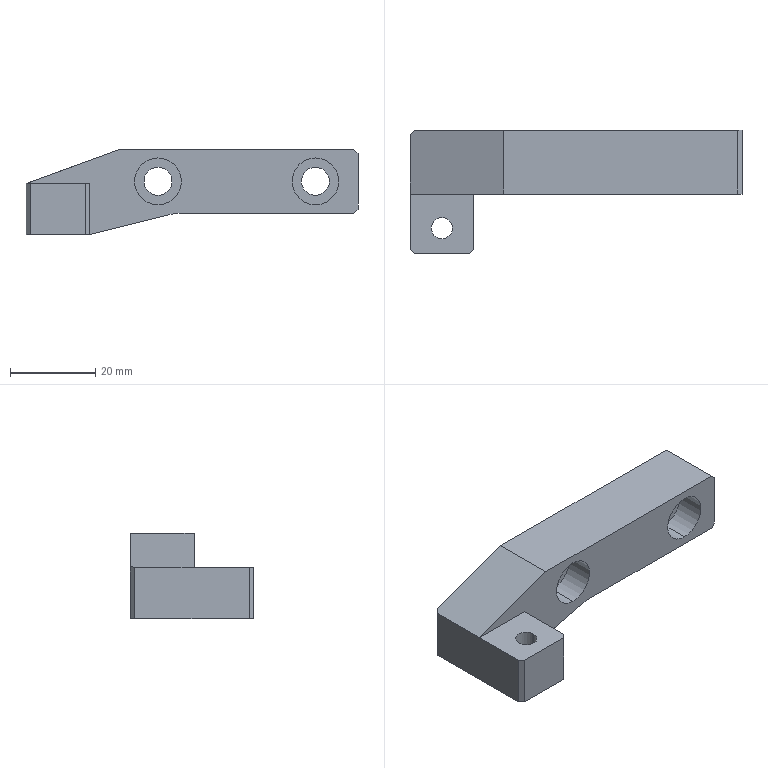Part | SolidWorks | features ICE 3, HoleWzd 2, Chamfer 1, Extrusion 1, Fillet 1 | 1 solid | 30 faces | box 78 x 29 x 20 mm | volume 18504 mm3 | plane 19 | cylinder 11 | commonest cylinder face diameters 6.6 x4 11 x4 5 x2 20 x1
STEP:
#1=CARTESIAN_POINT('',(-34.,-15.5,-12.5));
#2=VERTEX_POINT('',#1);
#3=CARTESIAN_POINT('',(-29.,-15.5,-12.5));
#4=VERTEX_POINT('',#3);
#5=CARTESIAN_POINT('',(-31.5,-15.5,-12.5));
#6=DIRECTION('',(0.,0.,1.));
#7=DIRECTION('',(1.,0.,0.));
#8=AXIS2_PLACEMENT_3D('',#5,#6,#7);
#9=CIRCLE('',#8,2.5);
#10=EDGE_CURVE('',#2,#4,#9,.T.);
#11=ORIENTED_EDGE('',*,*,#10,.F.);
#12=CARTESIAN_POINT('',(-34.,-15.5,-0.5));
#13=VERTEX_POINT('',#12);
#14=CARTESIAN_POINT('',(-34.,-15.5,-0.5));
#15=DIRECTION('',(0.,0.,1.));
#16=VECTOR('',#15,1000.);
#17=LINE('',#14,#16);
#18=EDGE_CURVE('',#2,#13,#17,.T.);
#19=ORIENTED_EDGE('',*,*,#18,.T.);
#20=CARTESIAN_POINT('',(-29.,-15.5,-0.5));
#21=VERTEX_POINT('',#20);
#22=CARTESIAN_POINT('',(-31.5,-15.5,-0.5));
#23=DIRECTION('',(0.,0.,1.));
#24=DIRECTION('',(1.,0.,0.));
#25=AXIS2_PLACEMENT_3D('',#22,#23,#24);
#26=CIRCLE('',#25,2.5);
#27=EDGE_CURVE('',#13,#21,#26,.T.);
#28=ORIENTED_EDGE('',*,*,#27,.T.);
#29=CARTESIAN_POINT('',(-29.,-15.5,-0.5));
#30=DIRECTION('',(0.,0.,1.));
#31=VECTOR('',#30,1000.);
#32=LINE('',#29,#31);
#33=EDGE_CURVE('',#4,#21,#32,.T.);
#34=ORIENTED_EDGE('',*,*,#33,.F.);
#35=EDGE_LOOP('',(#11,#19,#28,#34));
#36=FACE_OUTER_BOUND('',#35,.T.);
#37=CARTESIAN_POINT('',(-31.5,-15.5,-0.5));
#38=DIRECTION('',(0.,0.,1.));
#39=DIRECTION('',(1.,0.,0.));
#40=AXIS2_PLACEMENT_3D('',#37,#38,#39);
#41=CYLINDRICAL_SURFACE('',#40,2.5);
#42=ADVANCED_FACE('',(#36),#41,.F.);
#43=CARTESIAN_POINT('',(29.,-0.7,5.5));
#44=VERTEX_POINT('',#43);
#45=CARTESIAN_POINT('',(29.,-0.7,-5.5));
#46=VERTEX_POINT('',#45);
#47=CARTESIAN_POINT('',(29.,-0.7,0.));
#48=DIRECTION('',(0.,-1.,0.));
#49=DIRECTION('',(0.,0.,-1.));
#50=AXIS2_PLACEMENT_3D('',#47,#48,#49);
#51=CIRCLE('',#50,5.5);
#52=EDGE_CURVE('',#44,#46,#51,.T.);
#53=ORIENTED_EDGE('',*,*,#52,.F.);
#54=CARTESIAN_POINT('',(29.,-7.5,5.5));
#55=VERTEX_POINT('',#54);
#56=CARTESIAN_POINT('',(29.,-7.5,5.5));
#57=DIRECTION('',(0.,-1.,0.));
#58=VECTOR('',#57,1000.);
#59=LINE('',#56,#58);
#60=EDGE_CURVE('',#44,#55,#59,.T.);
#61=ORIENTED_EDGE('',*,*,#60,.T.);
#62=CARTESIAN_POINT('',(29.,-7.5,-5.5));
#63=VERTEX_POINT('',#62);
#64=CARTESIAN_POINT('',(29.,-7.5,0.));
#65=DIRECTION('',(0.,-1.,0.));
#66=DIRECTION('',(0.,0.,-1.));
#67=AXIS2_PLACEMENT_3D('',#64,#65,#66);
#68=CIRCLE('',#67,5.5);
#69=EDGE_CURVE('',#55,#63,#68,.T.);
#70=ORIENTED_EDGE('',*,*,#69,.T.);
#71=CARTESIAN_POINT('',(29.,-7.5,-5.5));
#72=DIRECTION('',(0.,-1.,0.));
#73=VECTOR('',#72,1000.);
#74=LINE('',#71,#73);
#75=EDGE_CURVE('',#46,#63,#74,.T.);
#76=ORIENTED_EDGE('',*,*,#75,.F.);
#77=EDGE_LOOP('',(#53,#61,#70,#76));
#78=FACE_OUTER_BOUND('',#77,.T.);
#79=CARTESIAN_POINT('',(29.,-7.5,0.));
#80=DIRECTION('',(0.,-1.,0.));
#81=DIRECTION('',(0.,0.,-1.));
#82=AXIS2_PLACEMENT_3D('',#79,#80,#81);
#83=CYLINDRICAL_SURFACE('',#82,5.5);
#84=ADVANCED_FACE('',(#78),#83,.F.);
#85=CARTESIAN_POINT('',(29.,7.5,3.3));
#86=VERTEX_POINT('',#85);
#87=CARTESIAN_POINT('',(29.,7.5,-3.3));
#88=VERTEX_POINT('',#87);
#89=CARTESIAN_POINT('',(29.,7.5,0.));
#90=DIRECTION('',(0.,-1.,0.));
#91=DIRECTION('',(0.,0.,-1.));
#92=AXIS2_PLACEMENT_3D('',#89,#90,#91);
#93=CIRCLE('',#92,3.3);
#94=EDGE_CURVE('',#86,#88,#93,.T.);
#95=ORIENTED_EDGE('',*,*,#94,.F.);
#96=CARTESIAN_POINT('',(29.,-0.7,3.3));
#97=VERTEX_POINT('',#96);
#98=CARTESIAN_POINT('',(29.,-7.5,3.3));
#99=DIRECTION('',(0.,-1.,0.));
#100=VECTOR('',#99,1000.);
#101=LINE('',#98,#100);
#102=EDGE_CURVE('',#86,#97,#101,.T.);
#103=ORIENTED_EDGE('',*,*,#102,.T.);
#104=CARTESIAN_POINT('',(29.,-0.7,-3.3));
#105=VERTEX_POINT('',#104);
#106=CARTESIAN_POINT('',(29.,-0.7,0.));
#107=DIRECTION('',(0.,-1.,0.));
#108=DIRECTION('',(0.,0.,-1.));
#109=AXIS2_PLACEMENT_3D('',#106,#107,#108);
#110=CIRCLE('',#109,3.3);
#111=EDGE_CURVE('',#97,#105,#110,.T.);
#112=ORIENTED_EDGE('',*,*,#111,.T.);
#113=CARTESIAN_POINT('',(29.,-7.5,-3.3));
#114=DIRECTION('',(0.,-1.,0.));
#115=VECTOR('',#114,1000.);
#116=LINE('',#113,#115);
#117=EDGE_CURVE('',#88,#105,#116,.T.);
#118=ORIENTED_EDGE('',*,*,#117,.F.);
#119=EDGE_LOOP('',(#95,#103,#112,#118));
#120=FACE_OUTER_BOUND('',#119,.T.);
#121=CARTESIAN_POINT('',(29.,-7.5,0.));
#122=DIRECTION('',(0.,-1.,0.));
#123=DIRECTION('',(0.,0.,-1.));
#124=AXIS2_PLACEMENT_3D('',#121,#122,#123);
#125=CYLINDRICAL_SURFACE('',#124,3.3);
#126=ADVANCED_FACE('',(#120),#125,.F.);
#127=CARTESIAN_POINT('',(-8.,-0.7,5.5));
#128=VERTEX_POINT('',#127);
#129=CARTESIAN_POINT('',(-8.,-0.7,-5.5));
#130=VERTEX_POINT('',#129);
#131=CARTESIAN_POINT('',(-8.,-0.7,0.));
#132=DIRECTION('',(0.,-1.,0.));
#133=DIRECTION('',(0.,0.,-1.));
#134=AXIS2_PLACEMENT_3D('',#131,#132,#133);
#135=CIRCLE('',#134,5.5);
#136=EDGE_CURVE('',#128,#130,#135,.T.);
#137=ORIENTED_EDGE('',*,*,#136,.F.);
#138=CARTESIAN_POINT('',(-8.,-7.5,5.5));
#139=VERTEX_POINT('',#138);
#140=CARTESIAN_POINT('',(-8.,-7.5,5.5));
#141=DIRECTION('',(0.,-1.,0.));
#142=VECTOR('',#141,1000.);
#143=LINE('',#140,#142);
#144=EDGE_CURVE('',#128,#139,#143,.T.);
#145=ORIENTED_EDGE('',*,*,#144,.T.);
#146=CARTESIAN_POINT('',(-8.,-7.5,-5.5));
#147=VERTEX_POINT('',#146);
#148=CARTESIAN_POINT('',(-8.,-7.5,0.));
#149=DIRECTION('',(0.,-1.,0.));
#150=DIRECTION('',(0.,0.,-1.));
#151=AXIS2_PLACEMENT_3D('',#148,#149,#150);
#152=CIRCLE('',#151,5.5);
#153=EDGE_CURVE('',#139,#147,#152,.T.);
#154=ORIENTED_EDGE('',*,*,#153,.T.);
#155=CARTESIAN_POINT('',(-8.,-7.5,-5.5));
#156=DIRECTION('',(0.,-1.,0.));
#157=VECTOR('',#156,1000.);
#158=LINE('',#155,#157);
#159=EDGE_CURVE('',#130,#147,#158,.T.);
#160=ORIENTED_EDGE('',*,*,#159,.F.);
#161=EDGE_LOOP('',(#137,#145,#154,#160));
#162=FACE_OUTER_BOUND('',#161,.T.);
#163=CARTESIAN_POINT('',(-8.,-7.5,0.));
#164=DIRECTION('',(0.,-1.,0.));
#165=DIRECTION('',(0.,0.,-1.));
#166=AXIS2_PLACEMENT_3D('',#163,#164,#165);
#167=CYLINDRICAL_SURFACE('',#166,5.5);
#168=ADVANCED_FACE('',(#162),#167,.F.);
#169=CARTESIAN_POINT('',(-8.,7.5,3.3));
#170=VERTEX_POINT('',#169);
#171=CARTESIAN_POINT('',(-8.,7.5,-3.3));
#172=VERTEX_POINT('',#171);
#173=CARTESIAN_POINT('',(-8.,7.5,0.));
#174=DIRECTION('',(0.,-1.,0.));
#175=DIRECTION('',(0.,0.,-1.));
#176=AXIS2_PLACEMENT_3D('',#173,#174,#175);
#177=CIRCLE('',#176,3.3);
#178=EDGE_CURVE('',#170,#172,#177,.T.);
#179=ORIENTED_EDGE('',*,*,#178,.F.);
#180=CARTESIAN_POINT('',(-8.,-0.7,3.3));
#181=VERTEX_POINT('',#180);
#182=CARTESIAN_POINT('',(-8.,-7.5,3.3));
#183=DIRECTION('',(0.,-1.,0.));
#184=VECTOR('',#183,1000.);
#185=LINE('',#182,#184);
#186=EDGE_CURVE('',#170,#181,#185,.T.);
#187=ORIENTED_EDGE('',*,*,#186,.T.);
#188=CARTESIAN_POINT('',(-8.,-0.7,-3.3));
#189=VERTEX_POINT('',#188);
#190=CARTESIAN_POINT('',(-8.,-0.7,0.));
#191=DIRECTION('',(0.,-1.,0.));
#192=DIRECTION('',(0.,0.,-1.));
#193=AXIS2_PLACEMENT_3D('',#190,#191,#192);
#194=CIRCLE('',#193,3.3);
#195=EDGE_CURVE('',#181,#189,#194,.T.);
#196=ORIENTED_EDGE('',*,*,#195,.T.);
#197=CARTESIAN_POINT('',(-8.,-7.5,-3.3));
#198=DIRECTION('',(0.,-1.,0.));
#199=VECTOR('',#198,1000.);
#200=LINE('',#197,#199);
#201=EDGE_CURVE('',#172,#189,#200,.T.);
#202=ORIENTED_EDGE('',*,*,#201,.F.);
#203=EDGE_LOOP('',(#179,#187,#196,#202));
#204=FACE_OUTER_BOUND('',#203,.T.);
#205=CARTESIAN_POINT('',(-8.,-7.5,0.));
#206=DIRECTION('',(0.,-1.,0.));
#207=DIRECTION('',(0.,0.,-1.));
#208=AXIS2_PLACEMENT_3D('',#205,#206,#207);
#209=CYLINDRICAL_SURFACE('',#208,3.3);
#210=ADVANCED_FACE('',(#204),#209,.F.);
#211=CARTESIAN_POINT('',(38.,-7.5,-7.5));
#212=VERTEX_POINT('',#211);
#213=CARTESIAN_POINT('',(-2.769,-7.5,-7.5));
#214=VERTEX_POINT('',#213);
#215=CARTESIAN_POINT('',(-39.,-7.5,-7.5));
#216=DIRECTION('',(-1.,0.,0.));
#217=VECTOR('',#216,1000.);
#218=LINE('',#215,#217);
#219=EDGE_CURVE('',#212,#214,#218,.T.);
#220=ORIENTED_EDGE('',*,*,#219,.F.);
#221=CARTESIAN_POINT('',(39.,-7.5,-6.5));
#222=VERTEX_POINT('',#221);
#223=CARTESIAN_POINT('',(22.75,-7.5,-22.75));
#224=DIRECTION('',(0.7071,0.,0.7071));
#225=VECTOR('',#224,1000.);
#226=LINE('',#223,#225);
#227=EDGE_CURVE('',#212,#222,#226,.T.);
#228=ORIENTED_EDGE('',*,*,#227,.T.);
#229=CARTESIAN_POINT('',(39.,-7.5,6.5));
#230=VERTEX_POINT('',#229);
#231=CARTESIAN_POINT('',(39.,-7.5,7.5));
#232=DIRECTION('',(0.,0.,-1.));
#233=VECTOR('',#232,1000.);
#234=LINE('',#231,#233);
#235=EDGE_CURVE('',#230,#222,#234,.T.);
#236=ORIENTED_EDGE('',*,*,#235,.F.);
#237=CARTESIAN_POINT('',(38.,-7.5,7.5));
#238=VERTEX_POINT('',#237);
#239=CARTESIAN_POINT('',(22.75,-7.5,22.75));
#240=DIRECTION('',(-0.7071,0.,0.7071));
#241=VECTOR('',#240,1000.);
#242=LINE('',#239,#241);
#243=EDGE_CURVE('',#230,#238,#242,.T.);
#244=ORIENTED_EDGE('',*,*,#243,.T.);
#245=CARTESIAN_POINT('',(-17.,-7.5,7.5));
#246=VERTEX_POINT('',#245);
#247=CARTESIAN_POINT('',(-39.,-7.5,7.5));
#248=DIRECTION('',(1.,0.,0.));
#249=VECTOR('',#248,1000.);
#250=LINE('',#247,#249);
#251=EDGE_CURVE('',#246,#238,#250,.T.);
#252=ORIENTED_EDGE('',*,*,#251,.F.);
#253=CARTESIAN_POINT('',(-39.,-7.5,-0.5));
#254=VERTEX_POINT('',#253);
#255=CARTESIAN_POINT('',(-4.394,-7.5,12.084));
#256=DIRECTION('',(0.9398,0.,0.3417));
#257=VECTOR('',#256,1000.);
#258=LINE('',#255,#257);
#259=EDGE_CURVE('',#254,#246,#258,.T.);
#260=ORIENTED_EDGE('',*,*,#259,.F.);
#261=CARTESIAN_POINT('',(-24.,-7.5,-0.5));
#262=VERTEX_POINT('',#261);
#263=CARTESIAN_POINT('',(-39.,-7.5,-0.5));
#264=DIRECTION('',(1.,0.,0.));
#265=VECTOR('',#264,1000.);
#266=LINE('',#263,#265);
#267=EDGE_CURVE('',#254,#262,#266,.T.);
#268=ORIENTED_EDGE('',*,*,#267,.T.);
#269=CARTESIAN_POINT('',(-24.,-7.5,-12.5));
#270=VERTEX_POINT('',#269);
#271=CARTESIAN_POINT('',(-24.,-7.5,-12.5));
#272=DIRECTION('',(0.,0.,-1.));
#273=VECTOR('',#272,1000.);
#274=LINE('',#271,#273);
#275=EDGE_CURVE('',#262,#270,#274,.T.);
#276=ORIENTED_EDGE('',*,*,#275,.T.);
#277=CARTESIAN_POINT('',(-5.194,-7.5,-7.799));
#278=VERTEX_POINT('',#277);
#279=CARTESIAN_POINT('',(-4.,-7.5,-7.5));
#280=DIRECTION('',(-0.9701,0.,-0.2425));
#281=VECTOR('',#280,1000.);
#282=LINE('',#279,#281);
#283=EDGE_CURVE('',#278,#270,#282,.T.);
#284=ORIENTED_EDGE('',*,*,#283,.F.);
#285=CARTESIAN_POINT('',(-2.769,-7.5,-17.5));
#286=DIRECTION('',(0.,1.,0.));
#287=DIRECTION('',(0.,0.,-1.));
#288=AXIS2_PLACEMENT_3D('',#285,#286,#287);
#289=CIRCLE('',#288,10.);
#290=EDGE_CURVE('',#278,#214,#289,.T.);
#291=ORIENTED_EDGE('',*,*,#290,.T.);
#292=EDGE_LOOP('',(#220,#228,#236,#244,#252,#260,#268,#276,#284,#291));
#293=FACE_OUTER_BOUND('',#292,.T.);
#294=CARTESIAN_POINT('',(29.,-7.5,0.));
#295=DIRECTION('',(0.,-1.,0.));
#296=DIRECTION('',(0.,0.,-1.));
#297=AXIS2_PLACEMENT_3D('',#294,#295,#296);
#298=CIRCLE('',#297,5.5);
#299=EDGE_CURVE('',#63,#55,#298,.T.);
#300=ORIENTED_EDGE('',*,*,#299,.F.);
#301=ORIENTED_EDGE('',*,*,#69,.F.);
#302=EDGE_LOOP('',(#300,#301));
#303=FACE_BOUND('',#302,.T.);
#304=CARTESIAN_POINT('',(-8.,-7.5,0.));
#305=DIRECTION('',(0.,-1.,0.));
#306=DIRECTION('',(0.,0.,-1.));
#307=AXIS2_PLACEMENT_3D('',#304,#305,#306);
#308=CIRCLE('',#307,5.5);
#309=EDGE_CURVE('',#147,#139,#308,.T.);
#310=ORIENTED_EDGE('',*,*,#309,.F.);
#311=ORIENTED_EDGE('',*,*,#153,.F.);
#312=EDGE_LOOP('',(#310,#311));
#313=FACE_BOUND('',#312,.T.);
#314=CARTESIAN_POINT('',(0.,-7.5,0.));
#315=DIRECTION('',(0.,-1.,0.));
#316=DIRECTION('',(0.,0.,-1.));
#317=AXIS2_PLACEMENT_3D('',#314,#315,#316);
#318=PLANE('',#317);
#319=ADVANCED_FACE('',(#293,#303,#313),#318,.T.);
#320=ORIENTED_EDGE('',*,*,#235,.T.);
#321=CARTESIAN_POINT('',(39.,7.5,-6.5));
#322=VERTEX_POINT('',#321);
#323=CARTESIAN_POINT('',(39.,7.5,-6.5));
#324=DIRECTION('',(0.,1.,0.));
#325=VECTOR('',#324,1000.);
#326=LINE('',#323,#325);
#327=EDGE_CURVE('',#222,#322,#326,.T.);
#328=ORIENTED_EDGE('',*,*,#327,.T.);
#329=CARTESIAN_POINT('',(39.,7.5,6.5));
#330=VERTEX_POINT('',#329);
#331=CARTESIAN_POINT('',(39.,7.5,7.5));
#332=DIRECTION('',(0.,0.,-1.));
#333=VECTOR('',#332,1000.);
#334=LINE('',#331,#333);
#335=EDGE_CURVE('',#330,#322,#334,.T.);
#336=ORIENTED_EDGE('',*,*,#335,.F.);
#337=CARTESIAN_POINT('',(39.,7.5,6.5));
#338=DIRECTION('',(0.,-1.,0.));
#339=VECTOR('',#338,1000.);
#340=LINE('',#337,#339);
#341=EDGE_CURVE('',#330,#230,#340,.T.);
#342=ORIENTED_EDGE('',*,*,#341,.T.);
#343=EDGE_LOOP('',(#320,#328,#336,#342));
#344=FACE_OUTER_BOUND('',#343,.T.);
#345=CARTESIAN_POINT('',(39.,7.5,7.5));
#346=DIRECTION('',(-1.,0.,0.));
#347=DIRECTION('',(0.,0.,1.));
#348=AXIS2_PLACEMENT_3D('',#345,#346,#347);
#349=PLANE('',#348);
#350=ADVANCED_FACE('',(#344),#349,.F.);
#351=ORIENTED_EDGE('',*,*,#219,.T.);
#352=CARTESIAN_POINT('',(-2.769,7.5,-7.5));
#353=VERTEX_POINT('',#352);
#354=CARTESIAN_POINT('',(-2.769,7.5,-7.5));
#355=DIRECTION('',(0.,1.,0.));
#356=VECTOR('',#355,1000.);
#357=LINE('',#354,#356);
#358=EDGE_CURVE('',#214,#353,#357,.T.);
#359=ORIENTED_EDGE('',*,*,#358,.T.);
#360=CARTESIAN_POINT('',(38.,7.5,-7.5));
#361=VERTEX_POINT('',#360);
#362=CARTESIAN_POINT('',(-39.,7.5,-7.5));
#363=DIRECTION('',(-1.,0.,0.));
#364=VECTOR('',#363,1000.);
#365=LINE('',#362,#364);
#366=EDGE_CURVE('',#361,#353,#365,.T.);
#367=ORIENTED_EDGE('',*,*,#366,.F.);
#368=CARTESIAN_POINT('',(38.,7.5,-7.5));
#369=DIRECTION('',(0.,-1.,0.));
#370=VECTOR('',#369,1000.);
#371=LINE('',#368,#370);
#372=EDGE_CURVE('',#361,#212,#371,.T.);
#373=ORIENTED_EDGE('',*,*,#372,.T.);
#374=EDGE_LOOP('',(#351,#359,#367,#373));
#375=FACE_OUTER_BOUND('',#374,.T.);
#376=CARTESIAN_POINT('',(-39.,7.5,-7.5));
#377=DIRECTION('',(0.,0.,1.));
#378=DIRECTION('',(1.,0.,0.));
#379=AXIS2_PLACEMENT_3D('',#376,#377,#378);
#380=PLANE('',#379);
#381=ADVANCED_FACE('',(#375),#380,.F.);
#382=CARTESIAN_POINT('',(-39.,6.5,-0.5));
#383=VERTEX_POINT('',#382);
#384=CARTESIAN_POINT('',(-39.,7.5,-0.5));
#385=DIRECTION('',(0.,-1.,0.));
#386=VECTOR('',#385,1000.);
#387=LINE('',#384,#386);
#388=EDGE_CURVE('',#383,#254,#387,.T.);
#389=ORIENTED_EDGE('',*,*,#388,.F.);
#390=CARTESIAN_POINT('',(-39.,6.5,-12.5));
#391=VERTEX_POINT('',#390);
#392=CARTESIAN_POINT('',(-39.,6.5,7.5));
#393=DIRECTION('',(0.,0.,-1.));
#394=VECTOR('',#393,1000.);
#395=LINE('',#392,#394);
#396=EDGE_CURVE('',#383,#391,#395,.T.);
#397=ORIENTED_EDGE('',*,*,#396,.T.);
#398=CARTESIAN_POINT('',(-39.,-20.5,-12.5));
#399=VERTEX_POINT('',#398);
#400=CARTESIAN_POINT('',(-39.,-42.855,-12.5));
#401=DIRECTION('',(0.,1.,0.));
#402=VECTOR('',#401,1000.);
#403=LINE('',#400,#402);
#404=EDGE_CURVE('',#399,#391,#403,.T.);
#405=ORIENTED_EDGE('',*,*,#404,.F.);
#406=CARTESIAN_POINT('',(-39.,-20.5,-0.5));
#407=VERTEX_POINT('',#406);
#408=CARTESIAN_POINT('',(-39.,-20.5,7.5));
#409=DIRECTION('',(0.,0.,1.));
#410=VECTOR('',#409,1000.);
#411=LINE('',#408,#410);
#412=EDGE_CURVE('',#399,#407,#411,.T.);
#413=ORIENTED_EDGE('',*,*,#412,.T.);
#414=CARTESIAN_POINT('',(-39.,-21.5,-0.5));
#415=DIRECTION('',(0.,1.,0.));
#416=VECTOR('',#415,1000.);
#417=LINE('',#414,#416);
#418=EDGE_CURVE('',#407,#254,#417,.T.);
#419=ORIENTED_EDGE('',*,*,#418,.T.);
#420=EDGE_LOOP('',(#389,#397,#405,#413,#419));
#421=FACE_OUTER_BOUND('',#420,.T.);
#422=CARTESIAN_POINT('',(-39.,7.5,7.5));
#423=DIRECTION('',(1.,0.,0.));
#424=DIRECTION('',(0.,0.,-1.));
#425=AXIS2_PLACEMENT_3D('',#422,#423,#424);
#426=PLANE('',#425);
#427=ADVANCED_FACE('',(#421),#426,.F.);
#428=ORIENTED_EDGE('',*,*,#251,.T.);
#429=CARTESIAN_POINT('',(38.,7.5,7.5));
#430=VERTEX_POINT('',#429);
#431=CARTESIAN_POINT('',(38.,7.5,7.5));
#432=DIRECTION('',(0.,1.,0.));
#433=VECTOR('',#432,1000.);
#434=LINE('',#431,#433);
#435=EDGE_CURVE('',#238,#430,#434,.T.);
#436=ORIENTED_EDGE('',*,*,#435,.T.);
#437=CARTESIAN_POINT('',(-17.,7.5,7.5));
#438=VERTEX_POINT('',#437);
#439=CARTESIAN_POINT('',(-39.,7.5,7.5));
#440=DIRECTION('',(1.,0.,0.));
#441=VECTOR('',#440,1000.);
#442=LINE('',#439,#441);
#443=EDGE_CURVE('',#438,#430,#442,.T.);
#444=ORIENTED_EDGE('',*,*,#443,.F.);
#445=CARTESIAN_POINT('',(-17.,7.5,7.5));
#446=DIRECTION('',(0.,-1.,0.));
#447=VECTOR('',#446,1000.);
#448=LINE('',#445,#447);
#449=EDGE_CURVE('',#438,#246,#448,.T.);
#450=ORIENTED_EDGE('',*,*,#449,.T.);
#451=EDGE_LOOP('',(#428,#436,#444,#450));
#452=FACE_OUTER_BOUND('',#451,.T.);
#453=CARTESIAN_POINT('',(-39.,7.5,7.5));
#454=DIRECTION('',(0.,0.,-1.));
#455=DIRECTION('',(-1.,0.,0.));
#456=AXIS2_PLACEMENT_3D('',#453,#454,#455);
#457=PLANE('',#456);
#458=ADVANCED_FACE('',(#452),#457,.F.);
#459=CARTESIAN_POINT('',(29.,7.5,0.));
#460=DIRECTION('',(0.,-1.,0.));
#461=DIRECTION('',(0.,0.,-1.));
#462=AXIS2_PLACEMENT_3D('',#459,#460,#461);
#463=CIRCLE('',#462,3.3);
#464=EDGE_CURVE('',#88,#86,#463,.T.);
#465=ORIENTED_EDGE('',*,*,#464,.T.);
#466=ORIENTED_EDGE('',*,*,#94,.T.);
#467=EDGE_LOOP('',(#465,#466));
#468=FACE_BOUND('',#467,.T.);
#469=CARTESIAN_POINT('',(-8.,7.5,0.));
#470=DIRECTION('',(0.,-1.,0.));
#471=DIRECTION('',(0.,0.,-1.));
#472=AXIS2_PLACEMENT_3D('',#469,#470,#471);
#473=CIRCLE('',#472,3.3);
#474=EDGE_CURVE('',#172,#170,#473,.T.);
#475=ORIENTED_EDGE('',*,*,#474,.T.);
#476=ORIENTED_EDGE('',*,*,#178,.T.);
#477=EDGE_LOOP('',(#475,#476));
#478=FACE_BOUND('',#477,.T.);
#479=CARTESIAN_POINT('',(-24.,7.5,-12.5));
#480=VERTEX_POINT('',#479);
#481=CARTESIAN_POINT('',(-38.,7.5,-12.5));
#482=VERTEX_POINT('',#481);
#483=CARTESIAN_POINT('',(-24.,7.5,-12.5));
#484=DIRECTION('',(-1.,0.,0.));
#485=VECTOR('',#484,1000.);
#486=LINE('',#483,#485);
#487=EDGE_CURVE('',#480,#482,#486,.T.);
#488=ORIENTED_EDGE('',*,*,#487,.T.);
#489=CARTESIAN_POINT('',(-38.,7.5,-0.1364));
#490=VERTEX_POINT('',#489);
#491=CARTESIAN_POINT('',(-38.,7.5,0.));
#492=DIRECTION('',(0.,0.,1.));
#493=VECTOR('',#492,1000.);
#494=LINE('',#491,#493);
#495=EDGE_CURVE('',#482,#490,#494,.T.);
#496=ORIENTED_EDGE('',*,*,#495,.T.);
#497=CARTESIAN_POINT('',(-39.,7.5,-0.5));
#498=DIRECTION('',(0.9398,0.,0.3417));
#499=VECTOR('',#498,1000.);
#500=LINE('',#497,#499);
#501=EDGE_CURVE('',#490,#438,#500,.T.);
#502=ORIENTED_EDGE('',*,*,#501,.T.);
#503=ORIENTED_EDGE('',*,*,#443,.T.);
#504=CARTESIAN_POINT('',(39.,7.5,6.5));
#505=DIRECTION('',(0.7071,0.,-0.7071));
#506=VECTOR('',#505,1000.);
#507=LINE('',#504,#506);
#508=EDGE_CURVE('',#430,#330,#507,.T.);
#509=ORIENTED_EDGE('',*,*,#508,.T.);
#510=ORIENTED_EDGE('',*,*,#335,.T.);
#511=CARTESIAN_POINT('',(38.,7.5,-7.5));
#512=DIRECTION('',(-0.7071,0.,-0.7071));
#513=VECTOR('',#512,1000.);
#514=LINE('',#511,#513);
#515=EDGE_CURVE('',#322,#361,#514,.T.);
#516=ORIENTED_EDGE('',*,*,#515,.T.);
#517=ORIENTED_EDGE('',*,*,#366,.T.);
#518=CARTESIAN_POINT('',(-5.194,7.5,-7.799));
#519=VERTEX_POINT('',#518);
#520=CARTESIAN_POINT('',(-2.769,7.5,-17.5));
#521=DIRECTION('',(0.,-1.,0.));
#522=DIRECTION('',(0.,0.,-1.));
#523=AXIS2_PLACEMENT_3D('',#520,#521,#522);
#524=CIRCLE('',#523,10.);
#525=EDGE_CURVE('',#353,#519,#524,.T.);
#526=ORIENTED_EDGE('',*,*,#525,.T.);
#527=CARTESIAN_POINT('',(-4.,7.5,-7.5));
#528=DIRECTION('',(-0.9701,0.,-0.2425));
#529=VECTOR('',#528,1000.);
#530=LINE('',#527,#529);
#531=EDGE_CURVE('',#519,#480,#530,.T.);
#532=ORIENTED_EDGE('',*,*,#531,.T.);
#533=EDGE_LOOP('',(#488,#496,#502,#503,#509,#510,#516,#517,#526,#532));
#534=FACE_OUTER_BOUND('',#533,.T.);
#535=CARTESIAN_POINT('',(0.,7.5,0.));
#536=DIRECTION('',(0.,-1.,0.));
#537=DIRECTION('',(0.,0.,-1.));
#538=AXIS2_PLACEMENT_3D('',#535,#536,#537);
#539=PLANE('',#538);
#540=ADVANCED_FACE('',(#468,#478,#534),#539,.F.);
#541=ORIENTED_EDGE('',*,*,#186,.F.);
#542=ORIENTED_EDGE('',*,*,#474,.F.);
#543=ORIENTED_EDGE('',*,*,#201,.T.);
#544=CARTESIAN_POINT('',(-8.,-0.7,0.));
#545=DIRECTION('',(0.,-1.,0.));
#546=DIRECTION('',(0.,0.,-1.));
#547=AXIS2_PLACEMENT_3D('',#544,#545,#546);
#548=CIRCLE('',#547,3.3);
#549=EDGE_CURVE('',#189,#181,#548,.T.);
#550=ORIENTED_EDGE('',*,*,#549,.T.);
#551=EDGE_LOOP('',(#541,#542,#543,#550));
#552=FACE_OUTER_BOUND('',#551,.T.);
#553=CARTESIAN_POINT('',(-8.,-7.5,0.));
#554=DIRECTION('',(0.,-1.,0.));
#555=DIRECTION('',(0.,0.,-1.));
#556=AXIS2_PLACEMENT_3D('',#553,#554,#555);
#557=CYLINDRICAL_SURFACE('',#556,3.3);
#558=ADVANCED_FACE('',(#552),#557,.F.);
#559=ORIENTED_EDGE('',*,*,#549,.F.);
#560=ORIENTED_EDGE('',*,*,#195,.F.);
#561=EDGE_LOOP('',(#559,#560));
#562=FACE_BOUND('',#561,.T.);
#563=CARTESIAN_POINT('',(-8.,-0.7,0.));
#564=DIRECTION('',(0.,-1.,0.));
#565=DIRECTION('',(0.,0.,-1.));
#566=AXIS2_PLACEMENT_3D('',#563,#564,#565);
#567=CIRCLE('',#566,5.5);
#568=EDGE_CURVE('',#130,#128,#567,.T.);
#569=ORIENTED_EDGE('',*,*,#568,.T.);
#570=ORIENTED_EDGE('',*,*,#136,.T.);
#571=EDGE_LOOP('',(#569,#570));
#572=FACE_OUTER_BOUND('',#571,.T.);
#573=CARTESIAN_POINT('',(-4.7,-0.7,0.));
#574=DIRECTION('',(0.,1.,0.));
#575=DIRECTION('',(0.,0.,1.));
#576=AXIS2_PLACEMENT_3D('',#573,#574,#575);
#577=PLANE('',#576);
#578=ADVANCED_FACE('',(#562,#572),#577,.F.);
#579=ORIENTED_EDGE('',*,*,#144,.F.);
#580=ORIENTED_EDGE('',*,*,#568,.F.);
#581=ORIENTED_EDGE('',*,*,#159,.T.);
#582=ORIENTED_EDGE('',*,*,#309,.T.);
#583=EDGE_LOOP('',(#579,#580,#581,#582));
#584=FACE_OUTER_BOUND('',#583,.T.);
#585=CARTESIAN_POINT('',(-8.,-7.5,0.));
#586=DIRECTION('',(0.,-1.,0.));
#587=DIRECTION('',(0.,0.,-1.));
#588=AXIS2_PLACEMENT_3D('',#585,#586,#587);
#589=CYLINDRICAL_SURFACE('',#588,5.5);
#590=ADVANCED_FACE('',(#584),#589,.F.);
#591=ORIENTED_EDGE('',*,*,#102,.F.);
#592=ORIENTED_EDGE('',*,*,#464,.F.);
#593=ORIENTED_EDGE('',*,*,#117,.T.);
#594=CARTESIAN_POINT('',(29.,-0.7,0.));
#595=DIRECTION('',(0.,-1.,0.));
#596=DIRECTION('',(0.,0.,-1.));
#597=AXIS2_PLACEMENT_3D('',#594,#595,#596);
#598=CIRCLE('',#597,3.3);
#599=EDGE_CURVE('',#105,#97,#598,.T.);
#600=ORIENTED_EDGE('',*,*,#599,.T.);
#601=EDGE_LOOP('',(#591,#592,#593,#600));
#602=FACE_OUTER_BOUND('',#601,.T.);
#603=CARTESIAN_POINT('',(29.,-7.5,0.));
#604=DIRECTION('',(0.,-1.,0.));
#605=DIRECTION('',(0.,0.,-1.));
#606=AXIS2_PLACEMENT_3D('',#603,#604,#605);
#607=CYLINDRICAL_SURFACE('',#606,3.3);
#608=ADVANCED_FACE('',(#602),#607,.F.);
#609=ORIENTED_EDGE('',*,*,#599,.F.);
#610=ORIENTED_EDGE('',*,*,#111,.F.);
#611=EDGE_LOOP('',(#609,#610));
#612=FACE_BOUND('',#611,.T.);
#613=CARTESIAN_POINT('',(29.,-0.7,0.));
#614=DIRECTION('',(0.,-1.,0.));
#615=DIRECTION('',(0.,0.,-1.));
#616=AXIS2_PLACEMENT_3D('',#613,#614,#615);
#617=CIRCLE('',#616,5.5);
#618=EDGE_CURVE('',#46,#44,#617,.T.);
#619=ORIENTED_EDGE('',*,*,#618,.T.);
#620=ORIENTED_EDGE('',*,*,#52,.T.);
#621=EDGE_LOOP('',(#619,#620));
#622=FACE_OUTER_BOUND('',#621,.T.);
#623=CARTESIAN_POINT('',(32.3,-0.7,0.));
#624=DIRECTION('',(0.,1.,0.));
#625=DIRECTION('',(0.,0.,1.));
#626=AXIS2_PLACEMENT_3D('',#623,#624,#625);
#627=PLANE('',#626);
#628=ADVANCED_FACE('',(#612,#622),#627,.F.);
#629=ORIENTED_EDGE('',*,*,#60,.F.);
#630=ORIENTED_EDGE('',*,*,#618,.F.);
#631=ORIENTED_EDGE('',*,*,#75,.T.);
#632=ORIENTED_EDGE('',*,*,#299,.T.);
#633=EDGE_LOOP('',(#629,#630,#631,#632));
#634=FACE_OUTER_BOUND('',#633,.T.);
#635=CARTESIAN_POINT('',(29.,-7.5,0.));
#636=DIRECTION('',(0.,-1.,0.));
#637=DIRECTION('',(0.,0.,-1.));
#638=AXIS2_PLACEMENT_3D('',#635,#636,#637);
#639=CYLINDRICAL_SURFACE('',#638,5.5);
#640=ADVANCED_FACE('',(#634),#639,.F.);
#641=CARTESIAN_POINT('',(-31.5,-15.5,-12.5));
#642=DIRECTION('',(0.,0.,1.));
#643=DIRECTION('',(1.,0.,0.));
#644=AXIS2_PLACEMENT_3D('',#641,#642,#643);
#645=CIRCLE('',#644,2.5);
#646=EDGE_CURVE('',#4,#2,#645,.T.);
#647=ORIENTED_EDGE('',*,*,#646,.T.);
#648=ORIENTED_EDGE('',*,*,#10,.T.);
#649=EDGE_LOOP('',(#647,#648));
#650=FACE_BOUND('',#649,.T.);
#651=ORIENTED_EDGE('',*,*,#404,.T.);
#652=CARTESIAN_POINT('',(-56.178,-10.678,-12.5));
#653=DIRECTION('',(0.7071,0.7071,0.));
#654=VECTOR('',#653,1000.);
#655=LINE('',#652,#654);
#656=EDGE_CURVE('',#391,#482,#655,.T.);
#657=ORIENTED_EDGE('',*,*,#656,.T.);
#658=ORIENTED_EDGE('',*,*,#487,.F.);
#659=CARTESIAN_POINT('',(-24.,-42.855,-12.5));
#660=DIRECTION('',(0.,1.,0.));
#661=VECTOR('',#660,1000.);
#662=LINE('',#659,#661);
#663=EDGE_CURVE('',#270,#480,#662,.T.);
#664=ORIENTED_EDGE('',*,*,#663,.F.);
#665=CARTESIAN_POINT('',(-24.,-20.5,-12.5));
#666=VERTEX_POINT('',#665);
#667=CARTESIAN_POINT('',(-24.,-21.5,-12.5));
#668=DIRECTION('',(0.,1.,0.));
#669=VECTOR('',#668,1000.);
#670=LINE('',#667,#669);
#671=EDGE_CURVE('',#666,#270,#670,.T.);
#672=ORIENTED_EDGE('',*,*,#671,.F.);
#673=CARTESIAN_POINT('',(-25.,-21.5,-12.5));
#674=VERTEX_POINT('',#673);
#675=CARTESIAN_POINT('',(-35.178,-31.678,-12.5));
#676=DIRECTION('',(-0.7071,-0.7071,0.));
#677=VECTOR('',#676,1000.);
#678=LINE('',#675,#677);
#679=EDGE_CURVE('',#666,#674,#678,.T.);
#680=ORIENTED_EDGE('',*,*,#679,.T.);
#681=CARTESIAN_POINT('',(-38.,-21.5,-12.5));
#682=VERTEX_POINT('',#681);
#683=CARTESIAN_POINT('',(-39.,-21.5,-12.5));
#684=DIRECTION('',(-1.,0.,0.));
#685=VECTOR('',#684,1000.);
#686=LINE('',#683,#685);
#687=EDGE_CURVE('',#674,#682,#686,.T.);
#688=ORIENTED_EDGE('',*,*,#687,.T.);
#689=CARTESIAN_POINT('',(-20.322,-39.178,-12.5));
#690=DIRECTION('',(-0.7071,0.7071,0.));
#691=VECTOR('',#690,1000.);
#692=LINE('',#689,#691);
#693=EDGE_CURVE('',#682,#399,#692,.T.);
#694=ORIENTED_EDGE('',*,*,#693,.T.);
#695=EDGE_LOOP('',(#651,#657,#658,#664,#672,#680,#688,#694));
#696=FACE_OUTER_BOUND('',#695,.T.);
#697=CARTESIAN_POINT('',(-24.,-42.855,-12.5));
#698=DIRECTION('',(0.,0.,-1.));
#699=DIRECTION('',(-1.,0.,0.));
#700=AXIS2_PLACEMENT_3D('',#697,#698,#699);
#701=PLANE('',#700);
#702=ADVANCED_FACE('',(#650,#696),#701,.T.);
#703=ORIENTED_EDGE('',*,*,#531,.F.);
#704=CARTESIAN_POINT('',(-5.194,-42.855,-7.799));
#705=DIRECTION('',(0.,-1.,0.));
#706=VECTOR('',#705,1000.);
#707=LINE('',#704,#706);
#708=EDGE_CURVE('',#519,#278,#707,.T.);
#709=ORIENTED_EDGE('',*,*,#708,.T.);
#710=ORIENTED_EDGE('',*,*,#283,.T.);
#711=ORIENTED_EDGE('',*,*,#663,.T.);
#712=EDGE_LOOP('',(#703,#709,#710,#711));
#713=FACE_OUTER_BOUND('',#712,.T.);
#714=CARTESIAN_POINT('',(-4.,-42.855,-7.5));
#715=DIRECTION('',(0.2425,0.,-0.9701));
#716=DIRECTION('',(-0.9701,0.,-0.2425));
#717=AXIS2_PLACEMENT_3D('',#714,#715,#716);
#718=PLANE('',#717);
#719=ADVANCED_FACE('',(#713),#718,.T.);
#720=CARTESIAN_POINT('',(-24.,-20.5,-0.5));
#721=VERTEX_POINT('',#720);
#722=CARTESIAN_POINT('',(-24.,-21.5,-0.5));
#723=DIRECTION('',(0.,1.,0.));
#724=VECTOR('',#723,1000.);
#725=LINE('',#722,#724);
#726=EDGE_CURVE('',#721,#262,#725,.T.);
#727=ORIENTED_EDGE('',*,*,#726,.F.);
#728=CARTESIAN_POINT('',(-24.,-20.5,-12.5));
#729=DIRECTION('',(0.,0.,-1.));
#730=VECTOR('',#729,1000.);
#731=LINE('',#728,#730);
#732=EDGE_CURVE('',#721,#666,#731,.T.);
#733=ORIENTED_EDGE('',*,*,#732,.T.);
#734=ORIENTED_EDGE('',*,*,#671,.T.);
#735=ORIENTED_EDGE('',*,*,#275,.F.);
#736=EDGE_LOOP('',(#727,#733,#734,#735));
#737=FACE_OUTER_BOUND('',#736,.T.);
#738=CARTESIAN_POINT('',(-24.,-21.5,-12.5));
#739=DIRECTION('',(1.,0.,0.));
#740=DIRECTION('',(0.,0.,-1.));
#741=AXIS2_PLACEMENT_3D('',#738,#739,#740);
#742=PLANE('',#741);
#743=ADVANCED_FACE('',(#737),#742,.T.);
#744=CARTESIAN_POINT('',(-31.5,-15.5,-0.5));
#745=DIRECTION('',(0.,0.,1.));
#746=DIRECTION('',(1.,0.,0.));
#747=AXIS2_PLACEMENT_3D('',#744,#745,#746);
#748=CIRCLE('',#747,2.5);
#749=EDGE_CURVE('',#21,#13,#748,.T.);
#750=ORIENTED_EDGE('',*,*,#749,.F.);
#751=ORIENTED_EDGE('',*,*,#27,.F.);
#752=EDGE_LOOP('',(#750,#751));
#753=FACE_BOUND('',#752,.T.);
#754=ORIENTED_EDGE('',*,*,#418,.F.);
#755=CARTESIAN_POINT('',(-38.,-21.5,-0.5));
#756=VERTEX_POINT('',#755);
#757=CARTESIAN_POINT('',(-38.5,-21.,-0.5));
#758=DIRECTION('',(0.7071,-0.7071,0.));
#759=VECTOR('',#758,1000.);
#760=LINE('',#757,#759);
#761=EDGE_CURVE('',#407,#756,#760,.T.);
#762=ORIENTED_EDGE('',*,*,#761,.T.);
#763=CARTESIAN_POINT('',(-25.,-21.5,-0.5));
#764=VERTEX_POINT('',#763);
#765=CARTESIAN_POINT('',(-39.,-21.5,-0.5));
#766=DIRECTION('',(1.,0.,0.));
#767=VECTOR('',#766,1000.);
#768=LINE('',#765,#767);
#769=EDGE_CURVE('',#756,#764,#768,.T.);
#770=ORIENTED_EDGE('',*,*,#769,.T.);
#771=CARTESIAN_POINT('',(-32.,-28.5,-0.5));
#772=DIRECTION('',(0.7071,0.7071,0.));
#773=VECTOR('',#772,1000.);
#774=LINE('',#771,#773);
#775=EDGE_CURVE('',#764,#721,#774,.T.);
#776=ORIENTED_EDGE('',*,*,#775,.T.);
#777=ORIENTED_EDGE('',*,*,#726,.T.);
#778=ORIENTED_EDGE('',*,*,#267,.F.);
#779=EDGE_LOOP('',(#754,#762,#770,#776,#777,#778));
#780=FACE_OUTER_BOUND('',#779,.T.);
#781=CARTESIAN_POINT('',(-39.,-21.5,-0.5));
#782=DIRECTION('',(0.,0.,1.));
#783=DIRECTION('',(1.,0.,0.));
#784=AXIS2_PLACEMENT_3D('',#781,#782,#783);
#785=PLANE('',#784);
#786=ADVANCED_FACE('',(#753,#780),#785,.T.);
#787=ORIENTED_EDGE('',*,*,#769,.F.);
#788=CARTESIAN_POINT('',(-38.,-21.5,0.));
#789=DIRECTION('',(0.,0.,-1.));
#790=VECTOR('',#789,1000.);
#791=LINE('',#788,#790);
#792=EDGE_CURVE('',#756,#682,#791,.T.);
#793=ORIENTED_EDGE('',*,*,#792,.T.);
#794=ORIENTED_EDGE('',*,*,#687,.F.);
#795=CARTESIAN_POINT('',(-25.,-21.5,-0.5));
#796=DIRECTION('',(0.,0.,1.));
#797=VECTOR('',#796,1000.);
#798=LINE('',#795,#797);
#799=EDGE_CURVE('',#674,#764,#798,.T.);
#800=ORIENTED_EDGE('',*,*,#799,.T.);
#801=EDGE_LOOP('',(#787,#793,#794,#800));
#802=FACE_OUTER_BOUND('',#801,.T.);
#803=CARTESIAN_POINT('',(0.,-21.5,0.));
#804=DIRECTION('',(0.,1.,0.));
#805=DIRECTION('',(0.,0.,1.));
#806=AXIS2_PLACEMENT_3D('',#803,#804,#805);
#807=PLANE('',#806);
#808=ADVANCED_FACE('',(#802),#807,.F.);
#809=ORIENTED_EDGE('',*,*,#18,.F.);
#810=ORIENTED_EDGE('',*,*,#646,.F.);
#811=ORIENTED_EDGE('',*,*,#33,.T.);
#812=ORIENTED_EDGE('',*,*,#749,.T.);
#813=EDGE_LOOP('',(#809,#810,#811,#812));
#814=FACE_OUTER_BOUND('',#813,.T.);
#815=CARTESIAN_POINT('',(-31.5,-15.5,-0.5));
#816=DIRECTION('',(0.,0.,1.));
#817=DIRECTION('',(1.,0.,0.));
#818=AXIS2_PLACEMENT_3D('',#815,#816,#817);
#819=CYLINDRICAL_SURFACE('',#818,2.5);
#820=ADVANCED_FACE('',(#814),#819,.F.);
#821=ORIENTED_EDGE('',*,*,#501,.F.);
#822=CARTESIAN_POINT('',(-37.977,7.523,-0.1279));
#823=DIRECTION('',(-0.6848,-0.6848,-0.249));
#824=VECTOR('',#823,1000.);
#825=LINE('',#822,#824);
#826=EDGE_CURVE('',#490,#383,#825,.T.);
#827=ORIENTED_EDGE('',*,*,#826,.T.);
#828=ORIENTED_EDGE('',*,*,#388,.T.);
#829=ORIENTED_EDGE('',*,*,#259,.T.);
#830=ORIENTED_EDGE('',*,*,#449,.F.);
#831=EDGE_LOOP('',(#821,#827,#828,#829,#830));
#832=FACE_OUTER_BOUND('',#831,.T.);
#833=CARTESIAN_POINT('',(-39.,7.5,-0.5));
#834=DIRECTION('',(0.3417,0.,-0.9398));
#835=DIRECTION('',(-0.9398,0.,-0.3417));
#836=AXIS2_PLACEMENT_3D('',#833,#834,#835);
#837=PLANE('',#836);
#838=ADVANCED_FACE('',(#832),#837,.F.);
#839=ORIENTED_EDGE('',*,*,#656,.F.);
#840=ORIENTED_EDGE('',*,*,#396,.F.);
#841=ORIENTED_EDGE('',*,*,#826,.F.);
#842=ORIENTED_EDGE('',*,*,#495,.F.);
#843=EDGE_LOOP('',(#839,#840,#841,#842));
#844=FACE_OUTER_BOUND('',#843,.T.);
#845=CARTESIAN_POINT('',(-38.,7.5,0.));
#846=DIRECTION('',(0.7071,-0.7071,0.));
#847=DIRECTION('',(0.,0.,1.));
#848=AXIS2_PLACEMENT_3D('',#845,#846,#847);
#849=PLANE('',#848);
#850=ADVANCED_FACE('',(#844),#849,.F.);
#851=ORIENTED_EDGE('',*,*,#693,.F.);
#852=ORIENTED_EDGE('',*,*,#792,.F.);
#853=ORIENTED_EDGE('',*,*,#761,.F.);
#854=ORIENTED_EDGE('',*,*,#412,.F.);
#855=EDGE_LOOP('',(#851,#852,#853,#854));
#856=FACE_OUTER_BOUND('',#855,.T.);
#857=CARTESIAN_POINT('',(-39.,-20.5,7.5));
#858=DIRECTION('',(0.7071,0.7071,0.));
#859=DIRECTION('',(0.,0.,1.));
#860=AXIS2_PLACEMENT_3D('',#857,#858,#859);
#861=PLANE('',#860);
#862=ADVANCED_FACE('',(#856),#861,.F.);
#863=ORIENTED_EDGE('',*,*,#775,.F.);
#864=ORIENTED_EDGE('',*,*,#799,.F.);
#865=ORIENTED_EDGE('',*,*,#679,.F.);
#866=ORIENTED_EDGE('',*,*,#732,.F.);
#867=EDGE_LOOP('',(#863,#864,#865,#866));
#868=FACE_OUTER_BOUND('',#867,.T.);
#869=CARTESIAN_POINT('',(-24.,-20.5,-12.5));
#870=DIRECTION('',(0.7071,-0.7071,0.));
#871=DIRECTION('',(0.,0.,1.));
#872=AXIS2_PLACEMENT_3D('',#869,#870,#871);
#873=PLANE('',#872);
#874=ADVANCED_FACE('',(#868),#873,.T.);
#875=ORIENTED_EDGE('',*,*,#515,.F.);
#876=ORIENTED_EDGE('',*,*,#327,.F.);
#877=ORIENTED_EDGE('',*,*,#227,.F.);
#878=ORIENTED_EDGE('',*,*,#372,.F.);
#879=EDGE_LOOP('',(#875,#876,#877,#878));
#880=FACE_OUTER_BOUND('',#879,.T.);
#881=CARTESIAN_POINT('',(38.,7.5,-7.5));
#882=DIRECTION('',(-0.7071,0.,0.7071));
#883=DIRECTION('',(0.,-1.,0.));
#884=AXIS2_PLACEMENT_3D('',#881,#882,#883);
#885=PLANE('',#884);
#886=ADVANCED_FACE('',(#880),#885,.F.);
#887=ORIENTED_EDGE('',*,*,#508,.F.);
#888=ORIENTED_EDGE('',*,*,#435,.F.);
#889=ORIENTED_EDGE('',*,*,#243,.F.);
#890=ORIENTED_EDGE('',*,*,#341,.F.);
#891=EDGE_LOOP('',(#887,#888,#889,#890));
#892=FACE_OUTER_BOUND('',#891,.T.);
#893=CARTESIAN_POINT('',(39.,7.5,6.5));
#894=DIRECTION('',(-0.7071,0.,-0.7071));
#895=DIRECTION('',(0.,-1.,0.));
#896=AXIS2_PLACEMENT_3D('',#893,#894,#895);
#897=PLANE('',#896);
#898=ADVANCED_FACE('',(#892),#897,.F.);
#899=ORIENTED_EDGE('',*,*,#290,.F.);
#900=ORIENTED_EDGE('',*,*,#708,.F.);
#901=ORIENTED_EDGE('',*,*,#525,.F.);
#902=ORIENTED_EDGE('',*,*,#358,.F.);
#903=EDGE_LOOP('',(#899,#900,#901,#902));
#904=FACE_OUTER_BOUND('',#903,.T.);
#905=CARTESIAN_POINT('',(-2.769,7.5,-17.5));
#906=DIRECTION('',(0.,1.,0.));
#907=DIRECTION('',(0.,0.,1.));
#908=AXIS2_PLACEMENT_3D('',#905,#906,#907);
#909=CYLINDRICAL_SURFACE('',#908,10.);
#910=ADVANCED_FACE('',(#904),#909,.F.);
#911=CLOSED_SHELL('',(#42,#84,#126,#168,#210,#319,#350,#381,#427,#458,#540,#558,#578,#590,#608,#628,#640,#702,#719,#743,#786,#808,#820,#838,#850,#862,#874,#886,#898,#910));
#912=MANIFOLD_SOLID_BREP('',#911);
#913=CARTESIAN_POINT('',(0.,0.,0.));
#914=DIRECTION('',(0.,0.,1.));
#915=DIRECTION('',(1.,0.,0.));
#916=AXIS2_PLACEMENT_3D('',#913,#914,#915);
#917=(LENGTH_UNIT()NAMED_UNIT(*)SI_UNIT(.MILLI.,.METRE.));
#918=UNCERTAINTY_MEASURE_WITH_UNIT(LENGTH_MEASURE(0.00001),#917,'','');
#919=(NAMED_UNIT(*)PLANE_ANGLE_UNIT()SI_UNIT($,.RADIAN.));
#920=(NAMED_UNIT(*)SI_UNIT($,.STERADIAN.)SOLID_ANGLE_UNIT());
#921=(GEOMETRIC_REPRESENTATION_CONTEXT(3)GLOBAL_UNCERTAINTY_ASSIGNED_CONTEXT((#918))GLOBAL_UNIT_ASSIGNED_CONTEXT((#917,#919,#920))REPRESENTATION_CONTEXT('',''));
#922=ADVANCED_BREP_SHAPE_REPRESENTATION('',(#912,#916),#921);